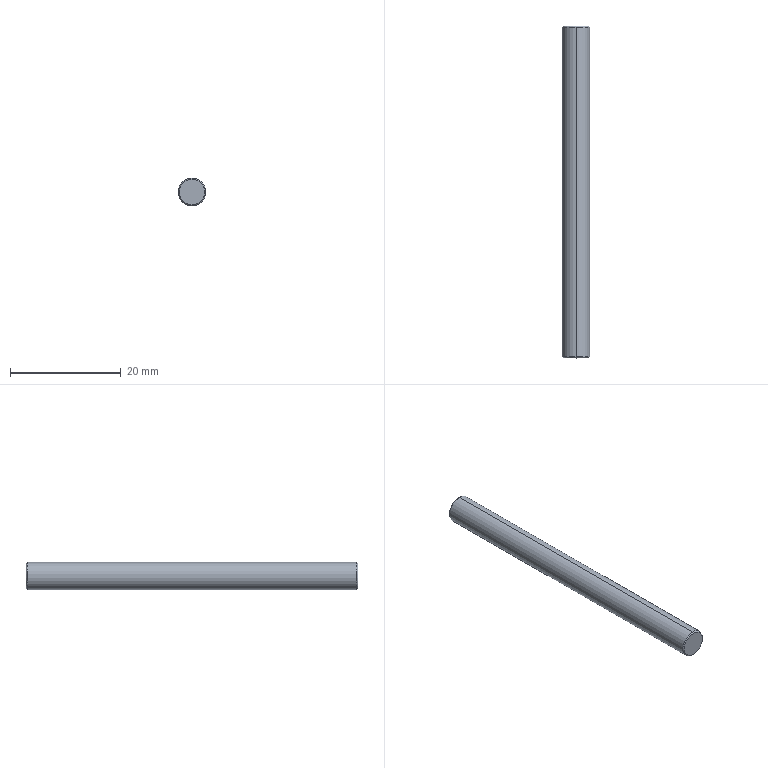Part | STEP file | 06-01-15 fibre mounting post | 1 solid | 12 faces | box 5 x 60 x 5 mm | volume 1139 mm3 | cone 6 | cylinder 4 | plane 2 | commonest cylinder face diameters 2.5 x2 5 x2
STEP:
#1=CARTESIAN_POINT('',(0.,52.5,-1.25));
#2=VERTEX_POINT('',#1);
#3=CARTESIAN_POINT('',(0.,52.5,1.25));
#4=VERTEX_POINT('',#3);
#5=CARTESIAN_POINT('',(0.,52.5,0.));
#6=DIRECTION('',(0.,1.,0.));
#7=DIRECTION('',(0.,0.,1.));
#8=AXIS2_PLACEMENT_3D('',#5,#6,#7);
#9=CIRCLE('',#8,1.25);
#10=EDGE_CURVE('',#2,#4,#9,.T.);
#11=ORIENTED_EDGE('',*,*,#10,.F.);
#12=CARTESIAN_POINT('',(0.,60.,-1.25));
#13=VERTEX_POINT('',#12);
#14=CARTESIAN_POINT('',(0.,60.,-1.25));
#15=DIRECTION('',(0.,1.,0.));
#16=VECTOR('',#15,1000.);
#17=LINE('',#14,#16);
#18=EDGE_CURVE('',#2,#13,#17,.T.);
#19=ORIENTED_EDGE('',*,*,#18,.T.);
#20=CARTESIAN_POINT('',(0.,60.,1.25));
#21=VERTEX_POINT('',#20);
#22=CARTESIAN_POINT('',(0.,60.,0.));
#23=DIRECTION('',(0.,1.,0.));
#24=DIRECTION('',(0.,0.,1.));
#25=AXIS2_PLACEMENT_3D('',#22,#23,#24);
#26=CIRCLE('',#25,1.25);
#27=EDGE_CURVE('',#13,#21,#26,.T.);
#28=ORIENTED_EDGE('',*,*,#27,.T.);
#29=CARTESIAN_POINT('',(0.,60.,1.25));
#30=DIRECTION('',(0.,1.,0.));
#31=VECTOR('',#30,1000.);
#32=LINE('',#29,#31);
#33=EDGE_CURVE('',#4,#21,#32,.T.);
#34=ORIENTED_EDGE('',*,*,#33,.F.);
#35=EDGE_LOOP('',(#11,#19,#28,#34));
#36=FACE_OUTER_BOUND('',#35,.T.);
#37=CARTESIAN_POINT('',(0.,60.,0.));
#38=DIRECTION('',(0.,1.,0.));
#39=DIRECTION('',(0.,0.,1.));
#40=AXIS2_PLACEMENT_3D('',#37,#38,#39);
#41=CYLINDRICAL_SURFACE('',#40,1.25);
#42=ADVANCED_FACE('',(#36),#41,.F.);
#43=CARTESIAN_POINT('',(0.,51.749,0.));
#44=VERTEX_POINT('',#43);
#45=CARTESIAN_POINT('',(0.,52.5,1.25));
#46=DIRECTION('',(0.,0.515,0.8572));
#47=VECTOR('',#46,1000.);
#48=LINE('',#45,#47);
#49=EDGE_CURVE('',#44,#4,#48,.T.);
#50=ORIENTED_EDGE('',*,*,#49,.F.);
#51=CARTESIAN_POINT('',(0.,52.5,-1.25));
#52=DIRECTION('',(0.,0.515,-0.8572));
#53=VECTOR('',#52,1000.);
#54=LINE('',#51,#53);
#55=EDGE_CURVE('',#44,#2,#54,.T.);
#56=ORIENTED_EDGE('',*,*,#55,.T.);
#57=ORIENTED_EDGE('',*,*,#10,.T.);
#58=EDGE_LOOP('',(#50,#56,#57));
#59=FACE_OUTER_BOUND('',#58,.T.);
#60=CARTESIAN_POINT('',(0.,52.5,0.));
#61=DIRECTION('',(0.,1.,0.));
#62=DIRECTION('',(0.,0.,1.));
#63=AXIS2_PLACEMENT_3D('',#60,#61,#62);
#64=CONICAL_SURFACE('',#63,1.25,1.03);
#65=ADVANCED_FACE('',(#59),#64,.F.);
#66=CARTESIAN_POINT('',(0.,60.,2.3));
#67=VERTEX_POINT('',#66);
#68=CARTESIAN_POINT('',(0.,60.,-2.3));
#69=VERTEX_POINT('',#68);
#70=CARTESIAN_POINT('',(0.,60.,0.));
#71=DIRECTION('',(0.,1.,0.));
#72=DIRECTION('',(0.,0.,1.));
#73=AXIS2_PLACEMENT_3D('',#70,#71,#72);
#74=CIRCLE('',#73,2.3);
#75=EDGE_CURVE('',#67,#69,#74,.T.);
#76=ORIENTED_EDGE('',*,*,#75,.F.);
#77=CARTESIAN_POINT('',(0.,59.8,2.5));
#78=VERTEX_POINT('',#77);
#79=CARTESIAN_POINT('',(0.,60.,2.3));
#80=DIRECTION('',(0.,-0.7071,0.7071));
#81=VECTOR('',#80,1000.);
#82=LINE('',#79,#81);
#83=EDGE_CURVE('',#67,#78,#82,.T.);
#84=ORIENTED_EDGE('',*,*,#83,.T.);
#85=CARTESIAN_POINT('',(0.,59.8,-2.5));
#86=VERTEX_POINT('',#85);
#87=CARTESIAN_POINT('',(0.,59.8,0.));
#88=DIRECTION('',(0.,-1.,0.));
#89=DIRECTION('',(0.,0.,1.));
#90=AXIS2_PLACEMENT_3D('',#87,#88,#89);
#91=CIRCLE('',#90,2.5);
#92=EDGE_CURVE('',#86,#78,#91,.T.);
#93=ORIENTED_EDGE('',*,*,#92,.F.);
#94=CARTESIAN_POINT('',(0.,60.,-2.3));
#95=DIRECTION('',(0.,-0.7071,-0.7071));
#96=VECTOR('',#95,1000.);
#97=LINE('',#94,#96);
#98=EDGE_CURVE('',#69,#86,#97,.T.);
#99=ORIENTED_EDGE('',*,*,#98,.F.);
#100=EDGE_LOOP('',(#76,#84,#93,#99));
#101=FACE_OUTER_BOUND('',#100,.T.);
#102=CARTESIAN_POINT('',(0.,60.,0.));
#103=DIRECTION('',(0.,-1.,0.));
#104=DIRECTION('',(0.,0.,-1.));
#105=AXIS2_PLACEMENT_3D('',#102,#103,#104);
#106=CONICAL_SURFACE('',#105,2.3,0.7854);
#107=ADVANCED_FACE('',(#101),#106,.T.);
#108=CARTESIAN_POINT('',(0.,0.,-2.3));
#109=VERTEX_POINT('',#108);
#110=CARTESIAN_POINT('',(0.,0.,2.3));
#111=VERTEX_POINT('',#110);
#112=CARTESIAN_POINT('',(0.,0.,0.));
#113=DIRECTION('',(0.,-1.,0.));
#114=DIRECTION('',(0.,0.,1.));
#115=AXIS2_PLACEMENT_3D('',#112,#113,#114);
#116=CIRCLE('',#115,2.3);
#117=EDGE_CURVE('',#109,#111,#116,.T.);
#118=ORIENTED_EDGE('',*,*,#117,.F.);
#119=CARTESIAN_POINT('',(0.,0.2,-2.5));
#120=VERTEX_POINT('',#119);
#121=CARTESIAN_POINT('',(0.,0.2,-2.5));
#122=DIRECTION('',(0.,0.7071,-0.7071));
#123=VECTOR('',#122,1000.);
#124=LINE('',#121,#123);
#125=EDGE_CURVE('',#109,#120,#124,.T.);
#126=ORIENTED_EDGE('',*,*,#125,.T.);
#127=CARTESIAN_POINT('',(0.,0.2,2.5));
#128=VERTEX_POINT('',#127);
#129=CARTESIAN_POINT('',(0.,0.2,0.));
#130=DIRECTION('',(0.,1.,0.));
#131=DIRECTION('',(0.,0.,1.));
#132=AXIS2_PLACEMENT_3D('',#129,#130,#131);
#133=CIRCLE('',#132,2.5);
#134=EDGE_CURVE('',#128,#120,#133,.T.);
#135=ORIENTED_EDGE('',*,*,#134,.F.);
#136=CARTESIAN_POINT('',(0.,0.2,2.5));
#137=DIRECTION('',(0.,0.7071,0.7071));
#138=VECTOR('',#137,1000.);
#139=LINE('',#136,#138);
#140=EDGE_CURVE('',#111,#128,#139,.T.);
#141=ORIENTED_EDGE('',*,*,#140,.F.);
#142=EDGE_LOOP('',(#118,#126,#135,#141));
#143=FACE_OUTER_BOUND('',#142,.T.);
#144=CARTESIAN_POINT('',(0.,0.2,0.));
#145=DIRECTION('',(0.,1.,0.));
#146=DIRECTION('',(0.,0.,1.));
#147=AXIS2_PLACEMENT_3D('',#144,#145,#146);
#148=CONICAL_SURFACE('',#147,2.5,0.7854);
#149=ADVANCED_FACE('',(#143),#148,.T.);
#150=ORIENTED_EDGE('',*,*,#92,.T.);
#151=CARTESIAN_POINT('',(0.,60.,2.5));
#152=DIRECTION('',(0.,-1.,0.));
#153=VECTOR('',#152,1000.);
#154=LINE('',#151,#153);
#155=EDGE_CURVE('',#78,#128,#154,.T.);
#156=ORIENTED_EDGE('',*,*,#155,.T.);
#157=ORIENTED_EDGE('',*,*,#134,.T.);
#158=CARTESIAN_POINT('',(0.,60.,-2.5));
#159=DIRECTION('',(0.,-1.,0.));
#160=VECTOR('',#159,1000.);
#161=LINE('',#158,#160);
#162=EDGE_CURVE('',#86,#120,#161,.T.);
#163=ORIENTED_EDGE('',*,*,#162,.F.);
#164=EDGE_LOOP('',(#150,#156,#157,#163));
#165=FACE_OUTER_BOUND('',#164,.T.);
#166=CARTESIAN_POINT('',(0.,60.,0.));
#167=DIRECTION('',(0.,-1.,0.));
#168=DIRECTION('',(0.,0.,-1.));
#169=AXIS2_PLACEMENT_3D('',#166,#167,#168);
#170=CYLINDRICAL_SURFACE('',#169,2.5);
#171=ADVANCED_FACE('',(#165),#170,.T.);
#172=ORIENTED_EDGE('',*,*,#155,.F.);
#173=CARTESIAN_POINT('',(0.,59.8,0.));
#174=DIRECTION('',(0.,-1.,0.));
#175=DIRECTION('',(0.,0.,1.));
#176=AXIS2_PLACEMENT_3D('',#173,#174,#175);
#177=CIRCLE('',#176,2.5);
#178=EDGE_CURVE('',#78,#86,#177,.T.);
#179=ORIENTED_EDGE('',*,*,#178,.T.);
#180=ORIENTED_EDGE('',*,*,#162,.T.);
#181=CARTESIAN_POINT('',(0.,0.2,0.));
#182=DIRECTION('',(0.,1.,0.));
#183=DIRECTION('',(0.,0.,1.));
#184=AXIS2_PLACEMENT_3D('',#181,#182,#183);
#185=CIRCLE('',#184,2.5);
#186=EDGE_CURVE('',#120,#128,#185,.T.);
#187=ORIENTED_EDGE('',*,*,#186,.T.);
#188=EDGE_LOOP('',(#172,#179,#180,#187));
#189=FACE_OUTER_BOUND('',#188,.T.);
#190=CARTESIAN_POINT('',(0.,60.,0.));
#191=DIRECTION('',(0.,-1.,0.));
#192=DIRECTION('',(0.,0.,-1.));
#193=AXIS2_PLACEMENT_3D('',#190,#191,#192);
#194=CYLINDRICAL_SURFACE('',#193,2.5);
#195=ADVANCED_FACE('',(#189),#194,.T.);
#196=CARTESIAN_POINT('',(0.,60.,0.));
#197=DIRECTION('',(0.,1.,0.));
#198=DIRECTION('',(0.,0.,1.));
#199=AXIS2_PLACEMENT_3D('',#196,#197,#198);
#200=CIRCLE('',#199,1.25);
#201=EDGE_CURVE('',#21,#13,#200,.T.);
#202=ORIENTED_EDGE('',*,*,#201,.F.);
#203=ORIENTED_EDGE('',*,*,#27,.F.);
#204=EDGE_LOOP('',(#202,#203));
#205=FACE_BOUND('',#204,.T.);
#206=CARTESIAN_POINT('',(0.,60.,0.));
#207=DIRECTION('',(0.,1.,0.));
#208=DIRECTION('',(0.,0.,1.));
#209=AXIS2_PLACEMENT_3D('',#206,#207,#208);
#210=CIRCLE('',#209,2.3);
#211=EDGE_CURVE('',#69,#67,#210,.T.);
#212=ORIENTED_EDGE('',*,*,#211,.T.);
#213=ORIENTED_EDGE('',*,*,#75,.T.);
#214=EDGE_LOOP('',(#212,#213));
#215=FACE_OUTER_BOUND('',#214,.T.);
#216=CARTESIAN_POINT('',(0.,60.,0.));
#217=DIRECTION('',(0.,1.,0.));
#218=DIRECTION('',(0.,0.,1.));
#219=AXIS2_PLACEMENT_3D('',#216,#217,#218);
#220=PLANE('',#219);
#221=ADVANCED_FACE('',(#205,#215),#220,.T.);
#222=CARTESIAN_POINT('',(0.,0.,0.));
#223=DIRECTION('',(0.,-1.,0.));
#224=DIRECTION('',(0.,0.,1.));
#225=AXIS2_PLACEMENT_3D('',#222,#223,#224);
#226=CIRCLE('',#225,2.3);
#227=EDGE_CURVE('',#111,#109,#226,.T.);
#228=ORIENTED_EDGE('',*,*,#227,.T.);
#229=ORIENTED_EDGE('',*,*,#117,.T.);
#230=EDGE_LOOP('',(#228,#229));
#231=FACE_OUTER_BOUND('',#230,.T.);
#232=CARTESIAN_POINT('',(0.,0.,0.));
#233=DIRECTION('',(0.,1.,0.));
#234=DIRECTION('',(0.,0.,1.));
#235=AXIS2_PLACEMENT_3D('',#232,#233,#234);
#236=PLANE('',#235);
#237=ADVANCED_FACE('',(#231),#236,.F.);
#238=ORIENTED_EDGE('',*,*,#125,.F.);
#239=ORIENTED_EDGE('',*,*,#227,.F.);
#240=ORIENTED_EDGE('',*,*,#140,.T.);
#241=ORIENTED_EDGE('',*,*,#186,.F.);
#242=EDGE_LOOP('',(#238,#239,#240,#241));
#243=FACE_OUTER_BOUND('',#242,.T.);
#244=CARTESIAN_POINT('',(0.,0.2,0.));
#245=DIRECTION('',(0.,1.,0.));
#246=DIRECTION('',(0.,0.,1.));
#247=AXIS2_PLACEMENT_3D('',#244,#245,#246);
#248=CONICAL_SURFACE('',#247,2.5,0.7854);
#249=ADVANCED_FACE('',(#243),#248,.T.);
#250=ORIENTED_EDGE('',*,*,#83,.F.);
#251=ORIENTED_EDGE('',*,*,#211,.F.);
#252=ORIENTED_EDGE('',*,*,#98,.T.);
#253=ORIENTED_EDGE('',*,*,#178,.F.);
#254=EDGE_LOOP('',(#250,#251,#252,#253));
#255=FACE_OUTER_BOUND('',#254,.T.);
#256=CARTESIAN_POINT('',(0.,60.,0.));
#257=DIRECTION('',(0.,-1.,0.));
#258=DIRECTION('',(0.,0.,-1.));
#259=AXIS2_PLACEMENT_3D('',#256,#257,#258);
#260=CONICAL_SURFACE('',#259,2.3,0.7854);
#261=ADVANCED_FACE('',(#255),#260,.T.);
#262=ORIENTED_EDGE('',*,*,#55,.F.);
#263=ORIENTED_EDGE('',*,*,#49,.T.);
#264=CARTESIAN_POINT('',(0.,52.5,0.));
#265=DIRECTION('',(0.,1.,0.));
#266=DIRECTION('',(0.,0.,1.));
#267=AXIS2_PLACEMENT_3D('',#264,#265,#266);
#268=CIRCLE('',#267,1.25);
#269=EDGE_CURVE('',#4,#2,#268,.T.);
#270=ORIENTED_EDGE('',*,*,#269,.T.);
#271=EDGE_LOOP('',(#262,#263,#270));
#272=FACE_OUTER_BOUND('',#271,.T.);
#273=CARTESIAN_POINT('',(0.,52.5,0.));
#274=DIRECTION('',(0.,1.,0.));
#275=DIRECTION('',(0.,0.,1.));
#276=AXIS2_PLACEMENT_3D('',#273,#274,#275);
#277=CONICAL_SURFACE('',#276,1.25,1.03);
#278=ADVANCED_FACE('',(#272),#277,.F.);
#279=ORIENTED_EDGE('',*,*,#18,.F.);
#280=ORIENTED_EDGE('',*,*,#269,.F.);
#281=ORIENTED_EDGE('',*,*,#33,.T.);
#282=ORIENTED_EDGE('',*,*,#201,.T.);
#283=EDGE_LOOP('',(#279,#280,#281,#282));
#284=FACE_OUTER_BOUND('',#283,.T.);
#285=CARTESIAN_POINT('',(0.,60.,0.));
#286=DIRECTION('',(0.,1.,0.));
#287=DIRECTION('',(0.,0.,1.));
#288=AXIS2_PLACEMENT_3D('',#285,#286,#287);
#289=CYLINDRICAL_SURFACE('',#288,1.25);
#290=ADVANCED_FACE('',(#284),#289,.F.);
#291=CLOSED_SHELL('',(#42,#65,#107,#149,#171,#195,#221,#237,#249,#261,#278,#290));
#292=MANIFOLD_SOLID_BREP('',#291);
#293=CARTESIAN_POINT('',(0.,0.,0.));
#294=DIRECTION('',(0.,0.,1.));
#295=DIRECTION('',(1.,0.,0.));
#296=AXIS2_PLACEMENT_3D('',#293,#294,#295);
#297=(LENGTH_UNIT()NAMED_UNIT(*)SI_UNIT(.MILLI.,.METRE.));
#298=UNCERTAINTY_MEASURE_WITH_UNIT(LENGTH_MEASURE(0.00001),#297,'','');
#299=(NAMED_UNIT(*)PLANE_ANGLE_UNIT()SI_UNIT($,.RADIAN.));
#300=(NAMED_UNIT(*)SI_UNIT($,.STERADIAN.)SOLID_ANGLE_UNIT());
#301=(GEOMETRIC_REPRESENTATION_CONTEXT(3)GLOBAL_UNCERTAINTY_ASSIGNED_CONTEXT((#298))GLOBAL_UNIT_ASSIGNED_CONTEXT((#297,#299,#300))REPRESENTATION_CONTEXT('',''));
#302=ADVANCED_BREP_SHAPE_REPRESENTATION('',(#292,#296),#301);